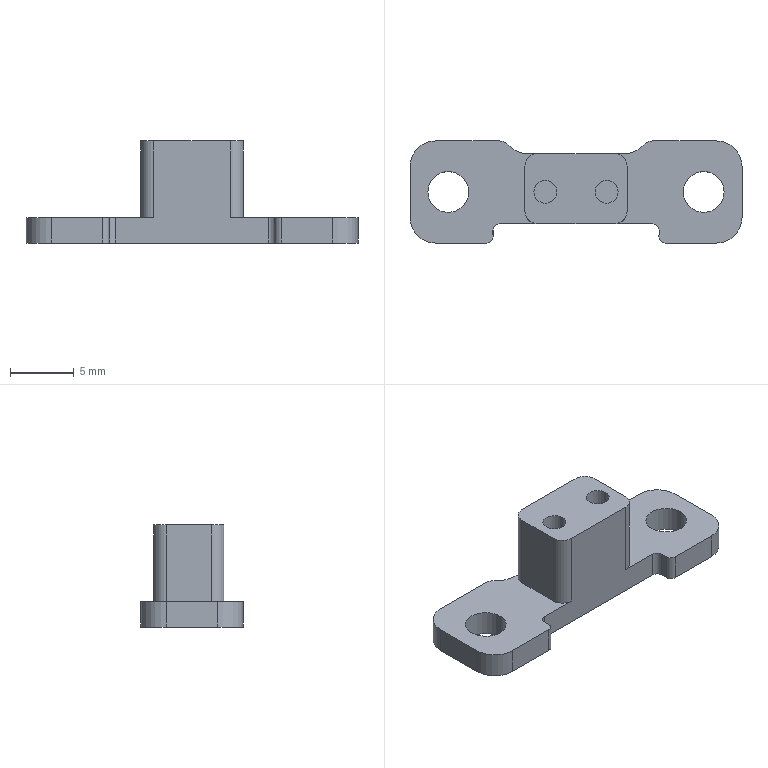NC program | Mastercam | posted with a generic post
Lines 11484 to 12913 of 12913:
(4 FEM |TOOL - 4|DIA. OFF. - 4|LEN. - 4|TOOL DIA. - 4.)
N3244 T4 M6
N3246 G0 G54 G90 X7.557 Y-6.8 C0. B0. S6000 M3
N3248 G43 H4 Z50.
N3250 Z-5.
N3252 G1 Z-6.3 F600.
N3254 Y-6.4 F1000.
N3256 G3 X7.157 Y-6. I-.4
N3258 G1 X7.
N3260 G2 X4.709 Y-4.5 J2.5
N3262 G1 X2.698
N3264 G3 X2.298 Y-4.9 J-.4
N3266 G1 Y-5.3
N3268 X7.557 Y-6.8
N3270 Z-6.6 F600.
N3272 Y-6.4 F1000.
N3274 G3 X7.157 Y-6. I-.4
N3276 G1 X7.
N3278 G2 X4.709 Y-4.5 J2.5
N3280 G1 X2.698
N3282 G3 X2.298 Y-4.9 J-.4
N3284 G1 Y-5.3
N3286 X7.557 Y-6.8
N3288 Z-6.9 F600.
N3290 Y-6.4 F1000.
N3292 G3 X7.157 Y-6. I-.4
N3294 G1 X7.
N3296 G2 X4.709 Y-4.5 J2.5
N3298 G1 X2.698
N3300 G3 X2.298 Y-4.9 J-.4
N3302 G1 Y-5.3
N3304 X7.557 Y-6.8
N3306 Z-7.2 F600.
N3308 Y-6.4 F1000.
N3310 G3 X7.157 Y-6. I-.4
N3312 G1 X7.
N3314 G2 X4.709 Y-4.5 J2.5
N3316 G1 X2.698
N3318 G3 X2.298 Y-4.9 J-.4
N3320 G1 Y-5.3
N3322 X7.557 Y-6.8
N3324 Z-7.5 F600.
N3326 Y-6.4 F1000.
N3328 G3 X7.157 Y-6. I-.4
N3330 G1 X7.
N3332 G2 X4.709 Y-4.5 J2.5
N3334 G1 X2.698
N3336 G3 X2.298 Y-4.9 J-.4
N3338 G1 Y-5.3
N3340 X7.557 Y-6.8
N3342 Z-7.8 F600.
N3344 Y-6.4 F1000.
N3346 G3 X7.157 Y-6. I-.4
N3348 G1 X7.
N3350 G2 X4.709 Y-4.5 J2.5
N3352 G1 X2.698
N3354 G3 X2.298 Y-4.9 J-.4
N3356 G1 Y-5.3
N3358 X7.557 Y-6.8
N3360 Z-8.1 F600.
N3362 Y-6.4 F1000.
N3364 G3 X7.157 Y-6. I-.4
N3366 G1 X7.
N3368 G2 X4.709 Y-4.5 J2.5
N3370 G1 X2.698
N3372 G3 X2.298 Y-4.9 J-.4
N3374 G1 Y-5.3
N3376 X7.557 Y-6.8
N3378 Z-8.4 F600.
N3380 Y-6.4 F1000.
N3382 G3 X7.157 Y-6. I-.4
N3384 G1 X7.
N3386 G2 X4.709 Y-4.5 J2.5
N3388 G1 X2.698
N3390 G3 X2.298 Y-4.9 J-.4
N3392 G1 Y-5.3
N3394 G0 Z50.
N3396 X-2.308
N3398 Z-5.
N3400 G1 Z-6.3 F600.
N3402 Y-4.9 F1000.
N3404 G3 X-2.708 Y-4.5 I-.4
N3406 G1 X-4.709
N3408 G2 X-7. Y-6. I-2.291 J1.
N3410 G1 X-7.182
N3412 G3 X-7.582 Y-6.4 J-.4
N3414 G1 Y-6.8
N3416 X-2.308 Y-5.3
N3418 Z-6.6 F600.
N3420 Y-4.9 F1000.
N3422 G3 X-2.708 Y-4.5 I-.4
N3424 G1 X-4.709
N3426 G2 X-7. Y-6. I-2.291 J1.
N3428 G1 X-7.182
N3430 G3 X-7.582 Y-6.4 J-.4
N3432 G1 Y-6.8
N3434 X-2.308 Y-5.3
N3436 Z-6.9 F600.
N3438 Y-4.9 F1000.
N3440 G3 X-2.708 Y-4.5 I-.4
N3442 G1 X-4.709
N3444 G2 X-7. Y-6. I-2.291 J1.
N3446 G1 X-7.182
N3448 G3 X-7.582 Y-6.4 J-.4
N3450 G1 Y-6.8
N3452 X-2.308 Y-5.3
N3454 Z-7.2 F600.
N3456 Y-4.9 F1000.
N3458 G3 X-2.708 Y-4.5 I-.4
N3460 G1 X-4.709
N3462 G2 X-7. Y-6. I-2.291 J1.
N3464 G1 X-7.182
N3466 G3 X-7.582 Y-6.4 J-.4
N3468 G1 Y-6.8
N3470 X-2.308 Y-5.3
N3472 Z-7.5 F600.
N3474 Y-4.9 F1000.
N3476 G3 X-2.708 Y-4.5 I-.4
N3478 G1 X-4.709
N3480 G2 X-7. Y-6. I-2.291 J1.
N3482 G1 X-7.182
N3484 G3 X-7.582 Y-6.4 J-.4
N3486 G1 Y-6.8
N3488 X-2.308 Y-5.3
N3490 Z-7.8 F600.
N3492 Y-4.9 F1000.
N3494 G3 X-2.708 Y-4.5 I-.4
N3496 G1 X-4.709
N3498 G2 X-7. Y-6. I-2.291 J1.
N3500 G1 X-7.182
N3502 G3 X-7.582 Y-6.4 J-.4
N3504 G1 Y-6.8
N3506 X-2.308 Y-5.3
N3508 Z-8.1 F600.
N3510 Y-4.9 F1000.
N3512 G3 X-2.708 Y-4.5 I-.4
N3514 G1 X-4.709
N3516 G2 X-7. Y-6. I-2.291 J1.
N3518 G1 X-7.182
N3520 G3 X-7.582 Y-6.4 J-.4
N3522 G1 Y-6.8
N3524 X-2.308 Y-5.3
N3526 Z-8.4 F600.
N3528 Y-4.9 F1000.
N3530 G3 X-2.708 Y-4.5 I-.4
N3532 G1 X-4.709
N3534 G2 X-7. Y-6. I-2.291 J1.
N3536 G1 X-7.182
N3538 G3 X-7.582 Y-6.4 J-.4
N3540 G1 Y-6.8
N3542 G0 Z50.
N3544 X-6.158 Y6.818
N3546 Z-5.
N3548 G1 Z-6.3 F600.
N3550 X-6.184 Y6.419 F1000.
N3552 G3 X-6.185 Y6.393 I.399 J-.026
N3554 X-5.81 Y5.994 I.4
N3556 G2 X-3.768 Y5. I-.194 J-2.994
N3558 G1 X-2.05
N3560 G3 X-1.65 Y5.4 J.4
N3562 G1 Y5.8
N3564 X-6.158 Y6.818
N3566 Z-6.6 F600.
N3568 X-6.184 Y6.419 F1000.
N3570 G3 X-6.185 Y6.393 I.399 J-.026
N3572 X-5.81 Y5.994 I.4
N3574 G2 X-3.768 Y5. I-.194 J-2.994
N3576 G1 X-2.05
N3578 G3 X-1.65 Y5.4 J.4
N3580 G1 Y5.8
N3582 X-6.158 Y6.818
N3584 Z-6.9 F600.
N3586 X-6.184 Y6.419 F1000.
N3588 G3 X-6.185 Y6.393 I.399 J-.026
N3590 X-5.81 Y5.994 I.4
N3592 G2 X-3.768 Y5. I-.194 J-2.994
N3594 G1 X-2.05
N3596 G3 X-1.65 Y5.4 J.4
N3598 G1 Y5.8
N3600 X-6.158 Y6.818
N3602 Z-7.2 F600.
N3604 X-6.184 Y6.419 F1000.
N3606 G3 X-6.185 Y6.393 I.399 J-.026
N3608 X-5.81 Y5.994 I.4
N3610 G2 X-3.768 Y5. I-.194 J-2.994
N3612 G1 X-2.05
N3614 G3 X-1.65 Y5.4 J.4
N3616 G1 Y5.8
N3618 X-6.158 Y6.818
N3620 Z-7.5 F600.
N3622 X-6.184 Y6.419 F1000.
N3624 G3 X-6.185 Y6.393 I.399 J-.026
N3626 X-5.81 Y5.994 I.4
N3628 G2 X-3.768 Y5. I-.194 J-2.994
N3630 G1 X-2.05
N3632 G3 X-1.65 Y5.4 J.4
N3634 G1 Y5.8
N3636 X-6.158 Y6.818
N3638 Z-7.8 F600.
N3640 X-6.184 Y6.419 F1000.
N3642 G3 X-6.185 Y6.393 I.399 J-.026
N3644 X-5.81 Y5.994 I.4
N3646 G2 X-3.768 Y5. I-.194 J-2.994
N3648 G1 X-2.05
N3650 G3 X-1.65 Y5.4 J.4
N3652 G1 Y5.8
N3654 X-6.158 Y6.818
N3656 Z-8.1 F600.
N3658 X-6.184 Y6.419 F1000.
N3660 G3 X-6.185 Y6.393 I.399 J-.026
N3662 X-5.81 Y5.994 I.4
N3664 G2 X-3.768 Y5. I-.194 J-2.994
N3666 G1 X-2.05
N3668 G3 X-1.65 Y5.4 J.4
N3670 G1 Y5.8
N3672 X-6.158 Y6.818
N3674 Z-8.4 F600.
N3676 X-6.184 Y6.419 F1000.
N3678 G3 X-6.185 Y6.393 I.399 J-.026
N3680 X-5.81 Y5.994 I.4
N3682 G2 X-3.768 Y5. I-.194 J-2.994
N3684 G1 X-2.05
N3686 G3 X-1.65 Y5.4 J.4
N3688 G1 Y5.8
N3690 G0 Z50.
N3692 X1.674
N3694 Z-5.
N3696 G1 Z-6.3 F600.
N3698 Y5.4 F1000.
N3700 G3 X2.074 Y5. I.4
N3702 G1 X3.768
N3704 G2 X5.81 Y5.994 I2.236 J-2.
N3706 G3 X6.185 Y6.393 I-.025 J.399
N3708 X6.184 Y6.419 I-.4
N3710 G1 X6.158 Y6.818
N3712 X1.674 Y5.8
N3714 Z-6.6 F600.
N3716 Y5.4 F1000.
N3718 G3 X2.074 Y5. I.4
N3720 G1 X3.768
N3722 G2 X5.81 Y5.994 I2.236 J-2.
N3724 G3 X6.185 Y6.393 I-.025 J.399
N3726 X6.184 Y6.419 I-.4
N3728 G1 X6.158 Y6.818
N3730 X1.674 Y5.8
N3732 Z-6.9 F600.
N3734 Y5.4 F1000.
N3736 G3 X2.074 Y5. I.4
N3738 G1 X3.768
N3740 G2 X5.81 Y5.994 I2.236 J-2.
N3742 G3 X6.185 Y6.393 I-.025 J.399
N3744 X6.184 Y6.419 I-.4
N3746 G1 X6.158 Y6.818
N3748 X1.674 Y5.8
N3750 Z-7.2 F600.
N3752 Y5.4 F1000.
N3754 G3 X2.074 Y5. I.4
N3756 G1 X3.768
N3758 G2 X5.81 Y5.994 I2.236 J-2.
N3760 G3 X6.185 Y6.393 I-.025 J.399
N3762 X6.184 Y6.419 I-.4
N3764 G1 X6.158 Y6.818
N3766 X1.674 Y5.8
N3768 Z-7.5 F600.
N3770 Y5.4 F1000.
N3772 G3 X2.074 Y5. I.4
N3774 G1 X3.768
N3776 G2 X5.81 Y5.994 I2.236 J-2.
N3778 G3 X6.185 Y6.393 I-.025 J.399
N3780 X6.184 Y6.419 I-.4
N3782 G1 X6.158 Y6.818
N3784 X1.674 Y5.8
N3786 Z-7.8 F600.
N3788 Y5.4 F1000.
N3790 G3 X2.074 Y5. I.4
N3792 G1 X3.768
N3794 G2 X5.81 Y5.994 I2.236 J-2.
N3796 G3 X6.185 Y6.393 I-.025 J.399
N3798 X6.184 Y6.419 I-.4
N3800 G1 X6.158 Y6.818
N3802 X1.674 Y5.8
N3804 Z-8.1 F600.
N3806 Y5.4 F1000.
N3808 G3 X2.074 Y5. I.4
N3810 G1 X3.768
N3812 G2 X5.81 Y5.994 I2.236 J-2.
N3814 G3 X6.185 Y6.393 I-.025 J.399
N3816 X6.184 Y6.419 I-.4
N3818 G1 X6.158 Y6.818
N3820 X1.674 Y5.8
N3822 Z-8.4 F600.
N3824 Y5.4 F1000.
N3826 G3 X2.074 Y5. I.4
N3828 G1 X3.768
N3830 G2 X5.81 Y5.994 I2.236 J-2.
N3832 G3 X6.185 Y6.393 I-.025 J.399
N3834 X6.184 Y6.419 I-.4
N3836 G1 X6.158 Y6.818
N3838 G0 Z50.
N3840 M5
N3842 G0 G28 G91 Z0.
N3844 G28
N3846 M01
N3848 G0 G17 G40 G80 G90 G94 G98
N3850 G0 G28 G91 Z0.
(1 FEM |TOOL - 1|DIA. OFF. - 1|LEN. - 1|TOOL DIA. - 1.)
N3852 T1 M6
N3854 G0 G54 G90 X6.193 Y-4.394 C0. B0. S6000 M3
N3856 G43 H1 Z50.
N3858 Z-5.
N3860 G1 Z-6.1 F600.
N3862 X6.266 Y-4.325 F500.
N3864 G3 X6.298 Y-4.252 I-.068 J.073
N3866 X6.27 Y-4.184 I-.1
N3868 G2 X6. Y-3.5 I.73 J.684
N3870 G1 Y-3.
N3872 X4.395
N3874 G3 X4.295 Y-3.1 J-.1
N3876 G1 Y-3.2
N3878 X6.193 Y-4.394
N3880 Z-6.2 F600.
N3882 X6.266 Y-4.325 F500.
N3884 G3 X6.298 Y-4.252 I-.068 J.073
N3886 X6.27 Y-4.184 I-.1
N3888 G2 X6. Y-3.5 I.73 J.684
N3890 G1 Y-3.
N3892 X4.395
N3894 G3 X4.295 Y-3.1 J-.1
N3896 G1 Y-3.2
N3898 X6.193 Y-4.394
N3900 Z-6.3 F600.
N3902 X6.266 Y-4.325 F500.
N3904 G3 X6.298 Y-4.252 I-.068 J.073
N3906 X6.27 Y-4.184 I-.1
N3908 G2 X6. Y-3.5 I.73 J.684
N3910 G1 Y-3.
N3912 X4.395
N3914 G3 X4.295 Y-3.1 J-.1
N3916 G1 Y-3.2
N3918 X6.193 Y-4.394
N3920 Z-6.4 F600.
N3922 X6.266 Y-4.325 F500.
N3924 G3 X6.298 Y-4.252 I-.068 J.073
N3926 X6.27 Y-4.184 I-.1
N3928 G2 X6. Y-3.5 I.73 J.684
N3930 G1 Y-3.
N3932 X4.395
N3934 G3 X4.295 Y-3.1 J-.1
N3936 G1 Y-3.2
N3938 X6.193 Y-4.394
N3940 Z-6.5 F600.
N3942 X6.266 Y-4.325 F500.
N3944 G3 X6.298 Y-4.252 I-.068 J.073
N3946 X6.27 Y-4.184 I-.1
N3948 G2 X6. Y-3.5 I.73 J.684
N3950 G1 Y-3.
N3952 X4.395
N3954 G3 X4.295 Y-3.1 J-.1
N3956 G1 Y-3.2
N3958 X6.193 Y-4.394
N3960 Z-6.6 F600.
N3962 X6.266 Y-4.325 F500.
N3964 G3 X6.298 Y-4.252 I-.068 J.073
N3966 X6.27 Y-4.184 I-.1
N3968 G2 X6. Y-3.5 I.73 J.684
N3970 G1 Y-3.
N3972 X4.395
N3974 G3 X4.295 Y-3.1 J-.1
N3976 G1 Y-3.2
N3978 X6.193 Y-4.394
N3980 Z-6.7 F600.
N3982 X6.266 Y-4.325 F500.
N3984 G3 X6.298 Y-4.252 I-.068 J.073
N3986 X6.27 Y-4.184 I-.1
N3988 G2 X6. Y-3.5 I.73 J.684
N3990 G1 Y-3.
N3992 X4.395
N3994 G3 X4.295 Y-3.1 J-.1
N3996 G1 Y-3.2
N3998 X6.193 Y-4.394
N4000 Z-6.8 F600.
N4002 X6.266 Y-4.325 F500.
N4004 G3 X6.298 Y-4.252 I-.068 J.073
N4006 X6.27 Y-4.184 I-.1
N4008 G2 X6. Y-3.5 I.73 J.684
N4010 G1 Y-3.
N4012 X4.395
N4014 G3 X4.295 Y-3.1 J-.1
N4016 G1 Y-3.2
N4018 X6.193 Y-4.394
N4020 Z-6.9 F600.
N4022 X6.266 Y-4.325 F500.
N4024 G3 X6.298 Y-4.252 I-.068 J.073
N4026 X6.27 Y-4.184 I-.1
N4028 G2 X6. Y-3.5 I.73 J.684
N4030 G1 Y-3.
N4032 X4.395
N4034 G3 X4.295 Y-3.1 J-.1
N4036 G1 Y-3.2
N4038 X6.193 Y-4.394
N4040 Z-7. F600.
N4042 X6.266 Y-4.325 F500.
N4044 G3 X6.298 Y-4.252 I-.068 J.073
N4046 X6.27 Y-4.184 I-.1
N4048 G2 X6. Y-3.5 I.73 J.684
N4050 G1 Y-3.
N4052 X4.395
N4054 G3 X4.295 Y-3.1 J-.1
N4056 G1 Y-3.2
N4058 X6.193 Y-4.394
N4060 Z-7.1 F600.
N4062 X6.266 Y-4.325 F500.
N4064 G3 X6.298 Y-4.252 I-.068 J.073
N4066 X6.27 Y-4.184 I-.1
N4068 G2 X6. Y-3.5 I.73 J.684
N4070 G1 Y-3.
N4072 X4.395
N4074 G3 X4.295 Y-3.1 J-.1
N4076 G1 Y-3.2
N4078 X6.193 Y-4.394
N4080 Z-7.2 F600.
N4082 X6.266 Y-4.325 F500.
N4084 G3 X6.298 Y-4.252 I-.068 J.073
N4086 X6.27 Y-4.184 I-.1
N4088 G2 X6. Y-3.5 I.73 J.684
N4090 G1 Y-3.
N4092 X4.395
N4094 G3 X4.295 Y-3.1 J-.1
N4096 G1 Y-3.2
N4098 X6.193 Y-4.394
N4100 Z-7.3 F600.
N4102 X6.266 Y-4.325 F500.
N4104 G3 X6.298 Y-4.252 I-.068 J.073
N4106 X6.27 Y-4.184 I-.1
N4108 G2 X6. Y-3.5 I.73 J.684
N4110 G1 Y-3.
N4112 X4.395
N4114 G3 X4.295 Y-3.1 J-.1
N4116 G1 Y-3.2
N4118 X6.193 Y-4.394
N4120 Z-7.4 F600.
N4122 X6.266 Y-4.325 F500.
N4124 G3 X6.298 Y-4.252 I-.068 J.073
N4126 X6.27 Y-4.184 I-.1
N4128 G2 X6. Y-3.5 I.73 J.684
N4130 G1 Y-3.
N4132 X4.395
N4134 G3 X4.295 Y-3.1 J-.1
N4136 G1 Y-3.2
N4138 X6.193 Y-4.394
N4140 Z-7.5 F600.
N4142 X6.266 Y-4.325 F500.
N4144 G3 X6.298 Y-4.252 I-.068 J.073
N4146 X6.27 Y-4.184 I-.1
N4148 G2 X6. Y-3.5 I.73 J.684
N4150 G1 Y-3.
N4152 X4.395
N4154 G3 X4.295 Y-3.1 J-.1
N4156 G1 Y-3.2
N4158 X6.193 Y-4.394
N4160 Z-7.6 F600.
N4162 X6.266 Y-4.325 F500.
N4164 G3 X6.298 Y-4.252 I-.068 J.073
N4166 X6.27 Y-4.184 I-.1
N4168 G2 X6. Y-3.5 I.73 J.684
N4170 G1 Y-3.
N4172 X4.395
N4174 G3 X4.295 Y-3.1 J-.1
N4176 G1 Y-3.2
N4178 X6.193 Y-4.394
N4180 Z-7.7 F600.
N4182 X6.266 Y-4.325 F500.
N4184 G3 X6.298 Y-4.252 I-.068 J.073
N4186 X6.27 Y-4.184 I-.1
N4188 G2 X6. Y-3.5 I.73 J.684
N4190 G1 Y-3.
N4192 X4.395
N4194 G3 X4.295 Y-3.1 J-.1
N4196 G1 Y-3.2
N4198 X6.193 Y-4.394
N4200 Z-7.8 F600.
N4202 X6.266 Y-4.325 F500.
N4204 G3 X6.298 Y-4.252 I-.068 J.073
N4206 X6.27 Y-4.184 I-.1
N4208 G2 X6. Y-3.5 I.73 J.684
N4210 G1 Y-3.
N4212 X4.395
N4214 G3 X4.295 Y-3.1 J-.1
N4216 G1 Y-3.2
N4218 X6.193 Y-4.394
N4220 Z-7.9 F600.
N4222 X6.266 Y-4.325 F500.
N4224 G3 X6.298 Y-4.252 I-.068 J.073
N4226 X6.27 Y-4.184 I-.1
N4228 G2 X6. Y-3.5 I.73 J.684
N4230 G1 Y-3.
N4232 X4.395
N4234 G3 X4.295 Y-3.1 J-.1
N4236 G1 Y-3.2
N4238 X6.193 Y-4.394
N4240 Z-8. F600.
N4242 X6.266 Y-4.325 F500.
N4244 G3 X6.298 Y-4.252 I-.068 J.073
N4246 X6.27 Y-4.184 I-.1
N4248 G2 X6. Y-3.5 I.73 J.684
N4250 G1 Y-3.
N4252 X4.395
N4254 G3 X4.295 Y-3.1 J-.1
N4256 G1 Y-3.2
N4258 X6.193 Y-4.394
N4260 Z-8.1 F600.
N4262 X6.266 Y-4.325 F500.
N4264 G3 X6.298 Y-4.252 I-.068 J.073
N4266 X6.27 Y-4.184 I-.1
N4268 G2 X6. Y-3.5 I.73 J.684
N4270 G1 Y-3.
N4272 X4.395
N4274 G3 X4.295 Y-3.1 J-.1
N4276 G1 Y-3.2
N4278 X6.193 Y-4.394
N4280 Z-8.2 F600.
N4282 X6.266 Y-4.325 F500.
N4284 G3 X6.298 Y-4.252 I-.068 J.073
N4286 X6.27 Y-4.184 I-.1
N4288 G2 X6. Y-3.5 I.73 J.684
N4290 G1 Y-3.
N4292 X4.395
N4294 G3 X4.295 Y-3.1 J-.1
N4296 G1 Y-3.2
N4298 X6.193 Y-4.394
N4300 Z-8.3 F600.
N4302 X6.266 Y-4.325 F500.
N4304 G3 X6.298 Y-4.252 I-.068 J.073
N4306 X6.27 Y-4.184 I-.1
N4308 G2 X6. Y-3.5 I.73 J.684
N4310 G1 Y-3.
N4312 X4.395
N4314 G3 X4.295 Y-3.1 J-.1
N4316 G1 Y-3.2
N4318 X6.193 Y-4.394
N4320 Z-8.4 F600.
N4322 X6.266 Y-4.325 F500.
N4324 G3 X6.298 Y-4.252 I-.068 J.073
N4326 X6.27 Y-4.184 I-.1
N4328 G2 X6. Y-3.5 I.73 J.684
N4330 G1 Y-3.
N4332 X4.395
N4334 G3 X4.295 Y-3.1 J-.1
N4336 G1 Y-3.2
N4338 G0 Z50.
N4340 X-4.296
N4342 Z-5.
N4344 G1 Z-6.1 F600.
N4346 Y-3.1 F500.
N4348 G3 X-4.396 Y-3. I-.1
N4350 G1 X-6.
N4352 Y-3.5
N4354 G2 X-6.27 Y-4.184 I-1.
N4356 G3 X-6.297 Y-4.252 I.072 J-.068
N4358 X-6.266 Y-4.325 I.099
N4360 G1 X-6.193 Y-4.394
N4362 X-4.296 Y-3.2
N4364 Z-6.2 F600.
N4366 Y-3.1 F500.
N4368 G3 X-4.396 Y-3. I-.1
N4370 G1 X-6.
N4372 Y-3.5
N4374 G2 X-6.27 Y-4.184 I-1.
N4376 G3 X-6.297 Y-4.252 I.072 J-.068
N4378 X-6.266 Y-4.325 I.099
N4380 G1 X-6.193 Y-4.394
N4382 X-4.296 Y-3.2
N4384 Z-6.3 F600.
N4386 Y-3.1 F500.
N4388 G3 X-4.396 Y-3. I-.1
N4390 G1 X-6.
N4392 Y-3.5
N4394 G2 X-6.27 Y-4.184 I-1.
N4396 G3 X-6.297 Y-4.252 I.072 J-.068
N4398 X-6.266 Y-4.325 I.099
N4400 G1 X-6.193 Y-4.394
N4402 X-4.296 Y-3.2
N4404 Z-6.4 F600.
N4406 Y-3.1 F500.
N4408 G3 X-4.396 Y-3. I-.1
N4410 G1 X-6.
N4412 Y-3.5
N4414 G2 X-6.27 Y-4.184 I-1.
N4416 G3 X-6.297 Y-4.252 I.072 J-.068
N4418 X-6.266 Y-4.325 I.099
N4420 G1 X-6.193 Y-4.394
N4422 X-4.296 Y-3.2
N4424 Z-6.5 F600.
N4426 Y-3.1 F500.
N4428 G3 X-4.396 Y-3. I-.1
N4430 G1 X-6.
N4432 Y-3.5
N4434 G2 X-6.27 Y-4.184 I-1.
N4436 G3 X-6.297 Y-4.252 I.072 J-.068
N4438 X-6.266 Y-4.325 I.099
N4440 G1 X-6.193 Y-4.394
N4442 X-4.296 Y-3.2
N4444 Z-6.6 F600.
N4446 Y-3.1 F500.
N4448 G3 X-4.396 Y-3. I-.1
N4450 G1 X-6.
N4452 Y-3.5
N4454 G2 X-6.27 Y-4.184 I-1.
N4456 G3 X-6.297 Y-4.252 I.072 J-.068
N4458 X-6.266 Y-4.325 I.099
N4460 G1 X-6.193 Y-4.394
N4462 X-4.296 Y-3.2
N4464 Z-6.7 F600.
N4466 Y-3.1 F500.
N4468 G3 X-4.396 Y-3. I-.1
N4470 G1 X-6.
N4472 Y-3.5
N4474 G2 X-6.27 Y-4.184 I-1.
N4476 G3 X-6.297 Y-4.252 I.072 J-.068
N4478 X-6.266 Y-4.325 I.099
N4480 G1 X-6.193 Y-4.394
N4482 X-4.296 Y-3.2
N4484 Z-6.8 F600.
N4486 Y-3.1 F500.
N4488 G3 X-4.396 Y-3. I-.1
N4490 G1 X-6.
N4492 Y-3.5
N4494 G2 X-6.27 Y-4.184 I-1.
N4496 G3 X-6.297 Y-4.252 I.072 J-.068
N4498 X-6.266 Y-4.325 I.099
N4500 G1 X-6.193 Y-4.394
N4502 X-4.296 Y-3.2
N4504 Z-6.9 F600.
N4506 Y-3.1 F500.
N4508 G3 X-4.396 Y-3. I-.1
N4510 G1 X-6.
N4512 Y-3.5
N4514 G2 X-6.27 Y-4.184 I-1.
N4516 G3 X-6.297 Y-4.252 I.072 J-.068
N4518 X-6.266 Y-4.325 I.099
N4520 G1 X-6.193 Y-4.394
N4522 X-4.296 Y-3.2
N4524 Z-7. F600.
N4526 Y-3.1 F500.
N4528 G3 X-4.396 Y-3. I-.1
N4530 G1 X-6.
N4532 Y-3.5
N4534 G2 X-6.27 Y-4.184 I-1.
N4536 G3 X-6.297 Y-4.252 I.072 J-.068
N4538 X-6.266 Y-4.325 I.099
N4540 G1 X-6.193 Y-4.394
N4542 X-4.296 Y-3.2
N4544 Z-7.1 F600.
N4546 Y-3.1 F500.
N4548 G3 X-4.396 Y-3. I-.1
N4550 G1 X-6.
N4552 Y-3.5
N4554 G2 X-6.27 Y-4.184 I-1.
N4556 G3 X-6.297 Y-4.252 I.072 J-.068
N4558 X-6.266 Y-4.325 I.099
N4560 G1 X-6.193 Y-4.394
N4562 X-4.296 Y-3.2
N4564 Z-7.2 F600.
N4566 Y-3.1 F500.
N4568 G3 X-4.396 Y-3. I-.1
N4570 G1 X-6.
N4572 Y-3.5
N4574 G2 X-6.27 Y-4.184 I-1.
N4576 G3 X-6.297 Y-4.252 I.072 J-.068
N4578 X-6.266 Y-4.325 I.099
N4580 G1 X-6.193 Y-4.394
N4582 X-4.296 Y-3.2
N4584 Z-7.3 F600.
N4586 Y-3.1 F500.
N4588 G3 X-4.396 Y-3. I-.1
N4590 G1 X-6.
N4592 Y-3.5
N4594 G2 X-6.27 Y-4.184 I-1.
N4596 G3 X-6.297 Y-4.252 I.072 J-.068
N4598 X-6.266 Y-4.325 I.099
N4600 G1 X-6.193 Y-4.394
N4602 X-4.296 Y-3.2
N4604 Z-7.4 F600.
N4606 Y-3.1 F500.
N4608 G3 X-4.396 Y-3. I-.1
N4610 G1 X-6.
N4612 Y-3.5
N4614 G2 X-6.27 Y-4.184 I-1.
N4616 G3 X-6.297 Y-4.252 I.072 J-.068
N4618 X-6.266 Y-4.325 I.099
N4620 G1 X-6.193 Y-4.394
N4622 X-4.296 Y-3.2
N4624 Z-7.5 F600.
N4626 Y-3.1 F500.
N4628 G3 X-4.396 Y-3. I-.1
N4630 G1 X-6.
N4632 Y-3.5
N4634 G2 X-6.27 Y-4.184 I-1.
N4636 G3 X-6.297 Y-4.252 I.072 J-.068
N4638 X-6.266 Y-4.325 I.099
N4640 G1 X-6.193 Y-4.394
N4642 X-4.296 Y-3.2
N4644 Z-7.6 F600.
N4646 Y-3.1 F500.
N4648 G3 X-4.396 Y-3. I-.1
N4650 G1 X-6.
N4652 Y-3.5
N4654 G2 X-6.27 Y-4.184 I-1.
N4656 G3 X-6.297 Y-4.252 I.072 J-.068
N4658 X-6.266 Y-4.325 I.099
N4660 G1 X-6.193 Y-4.394
N4662 X-4.296 Y-3.2
N4664 Z-7.7 F600.
N4666 Y-3.1 F500.
N4668 G3 X-4.396 Y-3. I-.1
N4670 G1 X-6.
N4672 Y-3.5
N4674 G2 X-6.27 Y-4.184 I-1.
N4676 G3 X-6.297 Y-4.252 I.072 J-.068
N4678 X-6.266 Y-4.325 I.099
N4680 G1 X-6.193 Y-4.394
N4682 X-4.296 Y-3.2
N4684 Z-7.8 F600.
N4686 Y-3.1 F500.
N4688 G3 X-4.396 Y-3. I-.1
N4690 G1 X-6.
N4692 Y-3.5
N4694 G2 X-6.27 Y-4.184 I-1.
N4696 G3 X-6.297 Y-4.252 I.072 J-.068
N4698 X-6.266 Y-4.325 I.099
N4700 G1 X-6.193 Y-4.394
N4702 X-4.296 Y-3.2
N4704 Z-7.9 F600.
N4706 Y-3.1 F500.
N4708 G3 X-4.396 Y-3. I-.1
N4710 G1 X-6.
N4712 Y-3.5
N4714 G2 X-6.27 Y-4.184 I-1.
N4716 G3 X-6.297 Y-4.252 I.072 J-.068
N4718 X-6.266 Y-4.325 I.099
N4720 G1 X-6.193 Y-4.394
N4722 X-4.296 Y-3.2
N4724 Z-8. F600.
N4726 Y-3.1 F500.
N4728 G3 X-4.396 Y-3. I-.1
N4730 G1 X-6.
N4732 Y-3.5
N4734 G2 X-6.27 Y-4.184 I-1.
N4736 G3 X-6.297 Y-4.252 I.072 J-.068
N4738 X-6.266 Y-4.325 I.099
N4740 G1 X-6.193 Y-4.394
N4742 X-4.296 Y-3.2
N4744 Z-8.1 F600.
N4746 Y-3.1 F500.
N4748 G3 X-4.396 Y-3. I-.1
N4750 G1 X-6.
N4752 Y-3.5
N4754 G2 X-6.27 Y-4.184 I-1.
N4756 G3 X-6.297 Y-4.252 I.072 J-.068
N4758 X-6.266 Y-4.325 I.099
N4760 G1 X-6.193 Y-4.394
N4762 X-4.296 Y-3.2
N4764 Z-8.2 F600.
N4766 Y-3.1 F500.
N4768 G3 X-4.396 Y-3. I-.1
N4770 G1 X-6.
N4772 Y-3.5
N4774 G2 X-6.27 Y-4.184 I-1.
N4776 G3 X-6.297 Y-4.252 I.072 J-.068
N4778 X-6.266 Y-4.325 I.099
N4780 G1 X-6.193 Y-4.394
N4782 X-4.296 Y-3.2
N4784 Z-8.3 F600.
N4786 Y-3.1 F500.
N4788 G3 X-4.396 Y-3. I-.1
N4790 G1 X-6.
N4792 Y-3.5
N4794 G2 X-6.27 Y-4.184 I-1.
N4796 G3 X-6.297 Y-4.252 I.072 J-.068
N4798 X-6.266 Y-4.325 I.099
N4800 G1 X-6.193 Y-4.394
N4802 X-4.296 Y-3.2
N4804 Z-8.4 F600.
N4806 Y-3.1 F500.
N4808 G3 X-4.396 Y-3. I-.1
N4810 G1 X-6.
N4812 Y-3.5
N4814 G2 X-6.27 Y-4.184 I-1.
N4816 G3 X-6.297 Y-4.252 I.072 J-.068
N4818 X-6.266 Y-4.325 I.099
N4820 G1 X-6.193 Y-4.394
N4822 G0 Z50.
N4824 M5
N4826 G0 G28 G91 Z0.
N4828 G28
N4830 M01
N4832 G0 G17 G40 G80 G90 G94 G98
N4834 G0 G28 G91 Z0.
(4 CHM |TOOL - 7|DIA. OFF. - 7|LEN. - 7|TOOL DIA. - 4.)
N4836 T7 M6
N4838 G0 G54 G90 X-10. Y0. C0. B0. S6000 M3
N4840 G43 H7 Z44.
N4842 G81 G98 Z-6.7 R-5. F200.
N4844 G80
N4846 Z50.
N4848 X-2.4
N4850 G81 G98 Z-.7 R1. F200.
N4852 X2.4
N4854 G80
N4856 X10.
N4858 Z44.
N4860 G81 G98 Z-6.7 R-5. F200.
N4862 G80
N4864 Z50.
N4866 X5.948 Y-.89
N4868 Z20.389
N4870 Z10.389
N4872 G1 Z.389 F600.
N4874 X5.936 Y-.889 Z.246 F1000.
N4876 X5.904 Y-.887 Z.104
N4878 X5.852 Y-.883 Z-.034
N4880 X5.786 Y-.878 Z-.168
N4882 X5.617 Y-.866 Z-.419
N4884 X5.419 Y-.852 Z-.641
N4886 X5.341 Y-.866 Z-.717
N4888 X5.268 Y-.916 Z-.786
N4890 X5.201 Y-.994 Z-.846
N4892 X5.141 Y-1.094 Z-.898
N4894 X5.09 Y-1.209 Z-.939
N4896 X5.049 Y-1.331 Z-.969
N4898 X5.019 Y-1.455 Z-.988
N4900 X5.003 Y-1.573 Z-.994
N4902 X4.985 Y-1.788
N4904 X4.924 Y-2.067
N4906 X4.824 Y-2.334
N4908 X4.688 Y-2.585
N4910 X4.516 Y-2.814
N4912 X4.314 Y-3.016
N4914 X4.085 Y-3.188
N4916 X3.834 Y-3.324
N4918 X3.567 Y-3.424
N4920 X3.288 Y-3.485
N4922 X3.037 Y-3.505
N4924 X2. Z-.995
N4926 X1.
N4928 X0.
N4930 X-1.
N4932 X-2.
N4934 X-3.037 Z-.994
N4936 X-3.288 Y-3.485
N4938 X-3.567 Y-3.424
N4940 X-3.834 Y-3.324
N4942 X-4.085 Y-3.187
N4944 X-4.314 Y-3.016
N4946 X-4.516 Y-2.814
N4948 X-4.687 Y-2.585
N4950 X-4.824 Y-2.334
N4952 X-4.924 Y-2.067
N4954 X-4.985 Y-1.788
N4956 X-5.005 Y-1.537
N4958 Y-.625 Z-.995
N4960 X-5.004 Y.25 Z-.996
N4962 X-5.005 Y1.125 Z-.995
N4964 Y2.037 Z-.994
N4966 X-4.985 Y2.288
N4968 X-4.924 Y2.567
N4970 X-4.824 Y2.834
N4972 X-4.687 Y3.085
N4974 X-4.516 Y3.314
N4976 X-4.314 Y3.516
N4978 X-4.085 Y3.687
N4980 X-3.834 Y3.824
N4982 X-3.567 Y3.924
N4984 X-3.288 Y3.985
N4986 X-3.037 Y4.005
N4988 X-2. Z-.995
N4990 X-1.
N4992 X0.
N4994 X1.
N4996 X2.
N4998 X3.037 Z-.994
N5000 X3.288 Y3.985
N5002 X3.567 Y3.924
N5004 X3.834 Y3.824
N5006 X4.085 Y3.688
N5008 X4.314 Y3.516
N5010 X4.516 Y3.314
N5012 X4.688 Y3.085
N5014 X4.824 Y2.834
N5016 X4.924 Y2.567
N5018 X4.985 Y2.288
N5020 X5.003 Y2.073
N5022 X5.005 Y2. Z-.995
N5024 Y1.125
N5026 Y.25
N5028 Y-.625
N5030 Y-1.5
N5032 X5.011 Y-1.618 Z-.989
N5034 X5.03 Y-1.744 Z-.97
N5036 X5.061 Y-1.869 Z-.939
N5038 X5.102 Y-1.988 Z-.898
N5040 X5.153 Y-2.092 Z-.847
N5042 X5.213 Y-2.175 Z-.787
N5044 X5.282 Y-2.23 Z-.718
N5046 X5.358 Y-2.25 Z-.642
N5048 X5.556 Z-.42
N5050 X5.726 Z-.169
N5052 X5.793 Z-.035
N5054 X5.844 Z.103
N5056 X5.877 Z.245
N5058 X5.889 Z.389
N5060 G0 Z10.389
N5062 Z20.389
N5064 Z50.
N5066 X4.364 Y5.059
N5068 Z13.929
N5070 Z3.929
N5072 G1 Z-6.071 F600.
N5074 X4.378 Y5.033 Z-6.261 F1000.
N5076 X4.414 Y4.963 Z-6.443
N5078 X4.467 Y4.863 Z-6.61
N5080 X4.528 Y4.746 Z-6.758
N5082 X4.563 Y4.708 Z-6.809
N5084 X4.616 Y4.685 Z-6.854
N5086 X4.684 Y4.675 Z-6.895
N5088 X4.761 Y4.678 Z-6.929
N5090 X4.927 Y4.712 Z-6.977
N5092 X5.078 Y4.773 Z-6.994
N5094 X5.186 Y4.831
N5096 X5.449 Y4.927
N5098 X5.72 Y4.985
N5100 X5.965 Y5.005
N5102 X7.003 Z-6.995
N5104 X8.002
N5106 X9.002
N5108 X10.001
N5110 X11.027
N5112 X11.316 Y4.988
N5114 X11.626 Y4.939
N5116 X11.93 Y4.857
N5118 X12.223 Y4.745
N5120 X12.502 Y4.603 Z-6.994
N5122 X12.766 Y4.431
N5124 X13.011 Y4.233
N5126 X13.233 Y4.011
N5128 X13.431 Y3.766
N5130 X13.603 Y3.502
N5132 X13.745 Y3.223 Z-6.995
N5134 X13.857 Y2.93
N5136 X13.939 Y2.626
N5138 X13.988 Y2.316
N5140 X14.004 Y2.054
N5142 X14.005 Y2.
N5144 Y1.
N5146 Y0.
N5148 Y-1.
N5150 Y-2.
N5152 X14.004 Y-2.054
N5154 X13.988 Y-2.316
N5156 X13.939 Y-2.626
N5158 X13.857 Y-2.93
N5160 X13.745 Y-3.223
N5162 X13.603 Y-3.502 Z-6.994
N5164 X13.431 Y-3.766
N5166 X13.233 Y-4.011
N5168 X13.011 Y-4.233
N5170 X12.766 Y-4.431
N5172 X12.502 Y-4.603
N5174 X12.223 Y-4.745 Z-6.995
N5176 X11.93 Y-4.857
N5178 X11.626 Y-4.939
N5180 X11.316 Y-4.988
N5182 X11.027 Y-5.005
N5184 X10.
N5186 X9.
N5188 X8.
N5190 X6.946 Z-6.994
N5192 X6.7 Y-4.976 Z-6.993
N5194 X6.423 Y-4.892
N5196 X6.163 Y-4.753
N5198 X5.935 Y-4.565
N5200 X5.747 Y-4.337
N5202 X5.616 Y-4.092
N5204 X5.523 Y-3.953 Z-6.977
N5206 X5.404 Y-3.828 Z-6.93
N5208 X5.34 Y-3.781 Z-6.896
N5210 X5.277 Y-3.749 Z-6.856
N5212 X5.218 Y-3.735 Z-6.809
N5214 X5.164 Y-3.744 Z-6.757
N5216 X5.043 Y-3.796 Z-6.609
N5218 X4.939 Y-3.84 Z-6.442
N5220 X4.866 Y-3.871 Z-6.261
N5222 X4.839 Y-3.883 Z-6.07
N5224 G0 Z3.93
N5226 Z13.93
N5228 Z50.
N5230 X-4.649 Y-4.391
N5232 Z14.393
N5234 Z4.393
N5236 G1 Z-5.607 F600.
N5238 X-4.658 Y-4.384 Z-5.751 F1000.
N5240 X-4.684 Y-4.364 Z-5.893
N5242 X-4.724 Y-4.332 Z-6.031
N5244 X-4.777 Y-4.291 Z-6.165
N5246 X-4.91 Y-4.187 Z-6.416
N5248 X-5.065 Y-4.065 Z-6.639
N5250 X-5.138 Y-4.033 Z-6.716
N5252 X-5.227 Z-6.785
N5254 X-5.327 Y-4.059 Z-6.845
N5256 X-5.433 Y-4.108 Z-6.896
N5258 X-5.541 Y-4.174 Z-6.938
N5260 X-5.644 Y-4.252 Z-6.968
N5262 X-5.739 Y-4.338 Z-6.987
N5264 X-5.819 Y-4.426 Z-6.993
N5266 X-5.935 Y-4.566
N5268 X-6.159 Y-4.751
N5270 X-6.419 Y-4.891
N5272 X-6.703 Y-4.977
N5274 X-6.949 Y-5.005 Z-6.994
N5276 X-8. Z-6.995
N5278 X-9.
N5280 X-10.
N5282 X-11.027
N5284 X-11.316 Y-4.988
N5286 X-11.626 Y-4.939
N5288 X-11.93 Y-4.857
N5290 X-12.223 Y-4.745
N5292 X-12.502 Y-4.603 Z-6.994
N5294 X-12.766 Y-4.431
N5296 X-13.011 Y-4.233
N5298 X-13.233 Y-4.011
N5300 X-13.431 Y-3.766
N5302 X-13.603 Y-3.502
N5304 X-13.745 Y-3.223 Z-6.995
N5306 X-13.857 Y-2.93
N5308 X-13.939 Y-2.626
N5310 X-13.988 Y-2.316
N5312 X-14.005 Y-2.027
N5314 Y-1.
N5316 Y0.
N5318 Y1.
N5320 Y2.027
N5322 X-13.988 Y2.316
N5324 X-13.939 Y2.626
N5326 X-13.857 Y2.93
N5328 X-13.745 Y3.223
N5330 X-13.603 Y3.502 Z-6.994
N5332 X-13.431 Y3.766
N5334 X-13.233 Y4.011
N5336 X-13.011 Y4.233
N5338 X-12.766 Y4.431
N5340 X-12.502 Y4.603
N5342 X-12.223 Y4.745 Z-6.995
N5344 X-11.93 Y4.857
N5346 X-11.626 Y4.939
N5348 X-11.316 Y4.988
N5350 X-11.027 Y5.005
N5352 X-10.001
N5354 X-9.002
N5356 X-8.002
N5358 X-7.003
N5360 X-5.965 Z-6.994
N5362 X-5.72 Y4.985
N5364 X-5.449 Y4.927
N5366 X-5.186 Y4.831
N5368 X-5.078 Y4.773
N5370 X-4.927 Y4.712 Z-6.977
N5372 X-4.761 Y4.678 Z-6.929
N5374 X-4.684 Y4.675 Z-6.895
N5376 X-4.616 Y4.685 Z-6.854
N5378 X-4.563 Y4.708 Z-6.809
N5380 X-4.528 Y4.746 Z-6.758
N5382 X-4.467 Y4.863 Z-6.61
N5384 X-4.414 Y4.963 Z-6.443
N5386 X-4.378 Y5.033 Z-6.261
N5388 X-4.364 Y5.059 Z-6.071
N5390 G0 Z3.929
N5392 Z13.929
N5394 Z50.
N5396 M5
N5398 G0 G28 G91 Z0.
N5400 G28
N5402 M01
N5404 G0 G17 G40 G80 G90 G94 G98
N5406 G0 G28 G91 Z0.
(6 FEM |TOOL - 6|DIA. OFF. - 6|LEN. - 6|TOOL DIA. - 6.)
N5408 T6 M6
N5410 G0 G54 G90 X-26.6 Y5.698 C0. B0. S8000 M3
N5412 G43 H6 Z57.
N5414 Z9.
N5416 G1 Z6.7 F600.
N5418 X23. F2000.
N5420 G2 X24.899 Y3.799 J-1.899
N5422 X23. Y1.899 I-1.899
N5424 G1 X-23.
N5426 G3 X-24.899 Y0. J-1.899
N5428 X-23. Y-1.899 I1.899
N5430 G1 X23.
N5432 G2 X24.9 Y-3.799 J-1.9
N5434 X23. Y-5.698 I-1.9
N5436 G1 X-26.6
N5438 G0 Z56.7
N5440 Y5.698
N5442 Z8.7
N5444 G1 Z6.4 F600.
N5446 X23. F2000.
N5448 G2 X24.899 Y3.799 J-1.899
N5450 X23. Y1.899 I-1.899
N5452 G1 X-23.
N5454 G3 X-24.899 Y0. J-1.899
N5456 X-23. Y-1.899 I1.899
N5458 G1 X23.
N5460 G2 X24.9 Y-3.799 J-1.9
N5462 X23. Y-5.698 I-1.9
N5464 G1 X-26.6
N5466 G0 Z56.4
N5468 Y5.698
N5470 Z8.4
N5472 G1 Z6.1 F600.
N5474 X23. F2000.
N5476 G2 X24.899 Y3.799 J-1.899
N5478 X23. Y1.899 I-1.899
N5480 G1 X-23.
N5482 G3 X-24.899 Y0. J-1.899
N5484 X-23. Y-1.899 I1.899
N5486 G1 X23.
N5488 G2 X24.9 Y-3.799 J-1.9
N5490 X23. Y-5.698 I-1.9
N5492 G1 X-26.6
N5494 G0 Z56.1
N5496 Y5.698
N5498 Z8.1
N5500 G1 Z5.8 F600.
N5502 X23. F2000.
N5504 G2 X24.899 Y3.799 J-1.899
N5506 X23. Y1.899 I-1.899
N5508 G1 X-23.
N5510 G3 X-24.899 Y0. J-1.899
N5512 X-23. Y-1.899 I1.899
N5514 G1 X23.
N5516 G2 X24.9 Y-3.799 J-1.9
N5518 X23. Y-5.698 I-1.9
N5520 G1 X-26.6
N5522 G0 Z55.8
N5524 Y5.698
N5526 Z7.8
N5528 G1 Z5.5 F600.
N5530 X23. F2000.
N5532 G2 X24.899 Y3.799 J-1.899
N5534 X23. Y1.899 I-1.899
N5536 G1 X-23.
N5538 G3 X-24.899 Y0. J-1.899
N5540 X-23. Y-1.899 I1.899
N5542 G1 X23.
N5544 G2 X24.9 Y-3.799 J-1.9
N5546 X23. Y-5.698 I-1.9
N5548 G1 X-26.6
N5550 G0 Z55.5
N5552 Y5.698
N5554 Z7.5
N5556 G1 Z5.2 F600.
N5558 X23. F2000.
N5560 G2 X24.899 Y3.799 J-1.899
N5562 X23. Y1.899 I-1.899
N5564 G1 X-23.
N5566 G3 X-24.899 Y0. J-1.899
N5568 X-23. Y-1.899 I1.899
N5570 G1 X23.
N5572 G2 X24.9 Y-3.799 J-1.9
N5574 X23. Y-5.698 I-1.9
N5576 G1 X-26.6
N5578 G0 Z55.2
N5580 Y5.698
N5582 Z7.2
N5584 G1 Z4.9 F600.
N5586 X23. F2000.
N5588 G2 X24.899 Y3.799 J-1.899
N5590 X23. Y1.899 I-1.899
N5592 G1 X-23.
N5594 G3 X-24.899 Y0. J-1.899
N5596 X-23. Y-1.899 I1.899
N5598 G1 X23.
N5600 G2 X24.9 Y-3.799 J-1.9
N5602 X23. Y-5.698 I-1.9
N5604 G1 X-26.6
N5606 G0 Z54.9
N5608 Y5.698
N5610 Z6.9
N5612 G1 Z4.6 F600.
N5614 X23. F2000.
N5616 G2 X24.899 Y3.799 J-1.899
N5618 X23. Y1.899 I-1.899
N5620 G1 X-23.
N5622 G3 X-24.899 Y0. J-1.899
N5624 X-23. Y-1.899 I1.899
N5626 G1 X23.
N5628 G2 X24.9 Y-3.799 J-1.9
N5630 X23. Y-5.698 I-1.9
N5632 G1 X-26.6
N5634 G0 Z54.6
N5636 Y5.698
N5638 Z6.6
N5640 G1 Z4.3 F600.
N5642 X23. F2000.
N5644 G2 X24.899 Y3.799 J-1.899
N5646 X23. Y1.899 I-1.899
N5648 G1 X-23.
N5650 G3 X-24.899 Y0. J-1.899
N5652 X-23. Y-1.899 I1.899
N5654 G1 X23.
N5656 G2 X24.9 Y-3.799 J-1.9
N5658 X23. Y-5.698 I-1.9
N5660 G1 X-26.6
N5662 G0 Z54.3
N5664 Y5.698
N5666 Z6.3
N5668 G1 Z4. F600.
N5670 X23. F2000.
N5672 G2 X24.899 Y3.799 J-1.899
N5674 X23. Y1.899 I-1.899
N5676 G1 X-23.
N5678 G3 X-24.899 Y0. J-1.899
N5680 X-23. Y-1.899 I1.899
N5682 G1 X23.
N5684 G2 X24.9 Y-3.799 J-1.9
N5686 X23. Y-5.698 I-1.9
N5688 G1 X-26.6
N5690 G0 Z54.
N5692 Y5.698
N5694 Z6.
N5696 G1 Z3.7 F600.
N5698 X23. F2000.
N5700 G2 X24.899 Y3.799 J-1.899
N5702 X23. Y1.899 I-1.899
N5704 G1 X-23.
N5706 G3 X-24.899 Y0. J-1.899
N5708 X-23. Y-1.899 I1.899
N5710 G1 X23.
N5712 G2 X24.9 Y-3.799 J-1.9
N5714 X23. Y-5.698 I-1.9
N5716 G1 X-26.6
N5718 G0 Z53.7
N5720 Y5.698
N5722 Z5.7
N5724 G1 Z3.4 F600.
N5726 X23. F2000.
N5728 G2 X24.899 Y3.799 J-1.899
N5730 X23. Y1.899 I-1.899
N5732 G1 X-23.
N5734 G3 X-24.899 Y0. J-1.899
N5736 X-23. Y-1.899 I1.899
N5738 G1 X23.
N5740 G2 X24.9 Y-3.799 J-1.9
N5742 X23. Y-5.698 I-1.9
N5744 G1 X-26.6
N5746 G0 Z53.4
N5748 Y5.698
N5750 Z5.4
N5752 G1 Z3.1 F600.
N5754 X23. F2000.
N5756 G2 X24.899 Y3.799 J-1.899
N5758 X23. Y1.899 I-1.899
N5760 G1 X-23.
N5762 G3 X-24.899 Y0. J-1.899
N5764 X-23. Y-1.899 I1.899
N5766 G1 X23.
N5768 G2 X24.9 Y-3.799 J-1.9
N5770 X23. Y-5.698 I-1.9
N5772 G1 X-26.6
N5774 G0 Z53.1
N5776 Y5.698
N5778 Z5.1
N5780 G1 Z2.8 F600.
N5782 X23. F2000.
N5784 G2 X24.899 Y3.799 J-1.899
N5786 X23. Y1.899 I-1.899
N5788 G1 X-23.
N5790 G3 X-24.899 Y0. J-1.899
N5792 X-23. Y-1.899 I1.899
N5794 G1 X23.
N5796 G2 X24.9 Y-3.799 J-1.9
N5798 X23. Y-5.698 I-1.9
N5800 G1 X-26.6
N5802 G0 Z52.8
N5804 Y5.698
N5806 Z4.8
N5808 G1 Z2.5 F600.
N5810 X23. F2000.
N5812 G2 X24.899 Y3.799 J-1.899
N5814 X23. Y1.899 I-1.899
N5816 G1 X-23.
N5818 G3 X-24.899 Y0. J-1.899
N5820 X-23. Y-1.899 I1.899
N5822 G1 X23.
N5824 G2 X24.9 Y-3.799 J-1.9
N5826 X23. Y-5.698 I-1.9
N5828 G1 X-26.6
N5830 G0 Z52.5
N5832 Y5.698
N5834 Z4.5
N5836 G1 Z2.2 F600.
N5838 X23. F2000.
N5840 G2 X24.899 Y3.799 J-1.899
N5842 X23. Y1.899 I-1.899
N5844 G1 X-23.
N5846 G3 X-24.899 Y0. J-1.899
N5848 X-23. Y-1.899 I1.899
N5850 G1 X23.
N5852 G2 X24.9 Y-3.799 J-1.9
N5854 X23. Y-5.698 I-1.9
N5856 G1 X-26.6
N5858 G0 Z52.2
N5860 Y5.698
N5862 Z4.2
N5864 G1 Z1.9 F600.
N5866 X23. F2000.
N5868 G2 X24.899 Y3.799 J-1.899
N5870 X23. Y1.899 I-1.899
N5872 G1 X-23.
N5874 G3 X-24.899 Y0. J-1.899
N5876 X-23. Y-1.899 I1.899
N5878 G1 X23.
N5880 G2 X24.9 Y-3.799 J-1.9
N5882 X23. Y-5.698 I-1.9
N5884 G1 X-26.6
N5886 G0 Z51.9
N5888 Y5.698
N5890 Z3.9
N5892 G1 Z1.6 F600.
N5894 X23. F2000.
N5896 G2 X24.899 Y3.799 J-1.899
N5898 X23. Y1.899 I-1.899
N5900 G1 X-23.
N5902 G3 X-24.899 Y0. J-1.899
N5904 X-23. Y-1.899 I1.899
N5906 G1 X23.
N5908 G2 X24.9 Y-3.799 J-1.9
N5910 X23. Y-5.698 I-1.9
N5912 G1 X-26.6
N5914 G0 Z51.6
N5916 Y5.698
N5918 Z3.6
N5920 G1 Z1.3 F600.
N5922 X23. F2000.
N5924 G2 X24.899 Y3.799 J-1.899
N5926 X23. Y1.899 I-1.899
N5928 G1 X-23.
N5930 G3 X-24.899 Y0. J-1.899
N5932 X-23. Y-1.899 I1.899
N5934 G1 X23.
N5936 G2 X24.9 Y-3.799 J-1.9
N5938 X23. Y-5.698 I-1.9
N5940 G1 X-26.6
N5942 G0 Z51.3
N5944 Y5.698
N5946 Z3.3
N5948 G1 Z1. F600.
N5950 X23. F2000.
N5952 G2 X24.899 Y3.799 J-1.899
N5954 X23. Y1.899 I-1.899
N5956 G1 X-23.
N5958 G3 X-24.899 Y0. J-1.899
N5960 X-23. Y-1.899 I1.899
N5962 G1 X23.
N5964 G2 X24.9 Y-3.799 J-1.9
N5966 X23. Y-5.698 I-1.9
N5968 G1 X-26.6
N5970 G0 Z51.
N5972 Y5.698
N5974 Z3.
N5976 G1 Z.7 F600.
N5978 X23. F2000.
N5980 G2 X24.899 Y3.799 J-1.899
N5982 X23. Y1.899 I-1.899
N5984 G1 X-23.
N5986 G3 X-24.899 Y0. J-1.899
N5988 X-23. Y-1.899 I1.899
N5990 G1 X23.
N5992 G2 X24.9 Y-3.799 J-1.9
N5994 X23. Y-5.698 I-1.9
N5996 G1 X-26.6
N5998 G0 Z50.7
N6000 Y5.698
N6002 Z2.7
N6004 G1 Z.4 F600.
N6006 X23. F2000.
N6008 G2 X24.899 Y3.799 J-1.899
N6010 X23. Y1.899 I-1.899
N6012 G1 X-23.
N6014 G3 X-24.899 Y0. J-1.899
N6016 X-23. Y-1.899 I1.899
N6018 G1 X23.
N6020 G2 X24.9 Y-3.799 J-1.9
N6022 X23. Y-5.698 I-1.9
N6024 G1 X-26.6
N6026 G0 Z50.4
N6028 Y5.698
N6030 Z2.4
N6032 G1 Z.1 F600.
N6034 X23. F2000.
N6036 G2 X24.899 Y3.799 J-1.899
N6038 X23. Y1.899 I-1.899
N6040 G1 X-23.
N6042 G3 X-24.899 Y0. J-1.899
N6044 X-23. Y-1.899 I1.899
N6046 G1 X23.
N6048 G2 X24.9 Y-3.799 J-1.9
N6050 X23. Y-5.698 I-1.9
N6052 G1 X-26.6
N6054 G0 Z50.1
N6056 Y5.698
N6058 Z2.1
N6060 G1 Z0. F600.
N6062 X23. F1000.
N6064 G2 X24.899 Y3.799 J-1.899
N6066 X23. Y1.899 I-1.899
N6068 G1 X-23.
N6070 G3 X-24.899 Y0. J-1.899
N6072 X-23. Y-1.899 I1.899
N6074 G1 X23.
N6076 G2 X24.9 Y-3.799 J-1.9
N6078 X23. Y-5.698 I-1.9
N6080 G1 X-26.6
N6082 G0 Z50.
N6084 M5
N6086 G0 G28 G91 Z0.
N6088 G0 G28 X0. Y0.
N6090 G28
N6092 M30
%